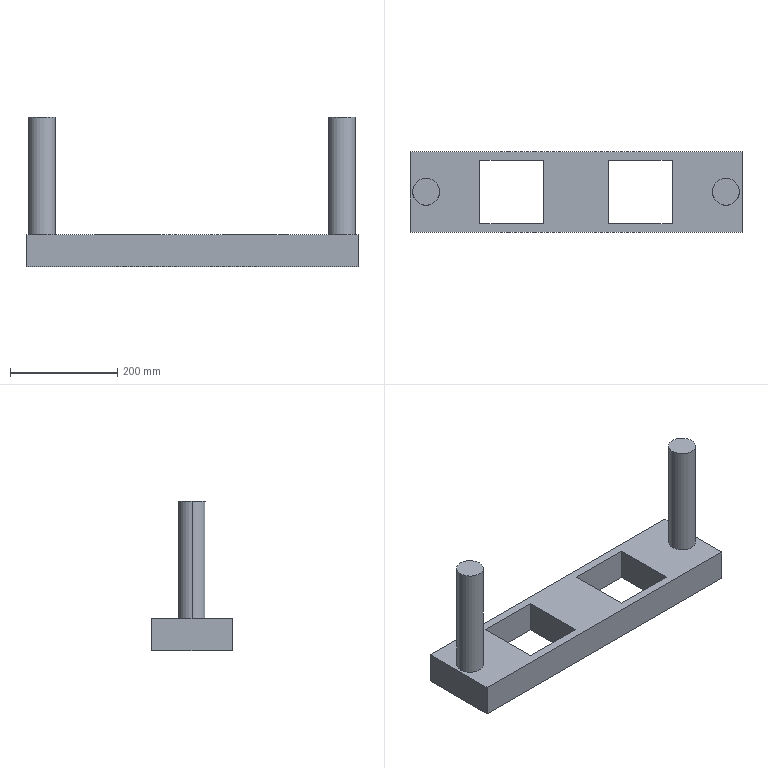Part | STEP file | 1 solid | 20 faces | box 620 x 150 x 280 mm | volume 4744618 mm3 | plane 16 | cylinder 4 | commonest cylinder face diameters 50 x4
STEP:
#1=CARTESIAN_POINT('',(0.,0.,0.));
#2=DIRECTION('',(0.,0.,1.));
#3=DIRECTION('',(1.,0.,0.));
#4=AXIS2_PLACEMENT_3D('',#1,#2,#3);
#5=CARTESIAN_POINT('',(-305.,0.,60.));
#6=VERTEX_POINT('',#5);
#7=CARTESIAN_POINT('',(-255.,0.,60.));
#8=VERTEX_POINT('',#7);
#9=CARTESIAN_POINT('',(-280.,0.,60.));
#10=DIRECTION('',(0.,0.,-1.));
#11=DIRECTION('',(1.,0.,0.));
#12=AXIS2_PLACEMENT_3D('',#9,#10,#11);
#13=CIRCLE('',#12,25.);
#14=CARTESIAN_POINT('',(-280.,0.,280.));
#15=DIRECTION('',(0.,0.,1.));
#16=DIRECTION('',(1.,0.,0.));
#17=AXIS2_PLACEMENT_3D('',#14,#15,#16);
#18=CYLINDRICAL_SURFACE('',#17,25.);
#19=CARTESIAN_POINT('',(6.283,-220.));
#20=DIRECTION('',(-1.,0.));
#21=VECTOR('',#20,1.);
#22=LINE('',#19,#21);
#23=(GEOMETRIC_REPRESENTATION_CONTEXT(2)PARAMETRIC_REPRESENTATION_CONTEXT()REPRESENTATION_CONTEXT('',''));
#24=DEFINITIONAL_REPRESENTATION('',(#22),#23);
#25=PCURVE('',#18,#24);
#26=CARTESIAN_POINT('',(0.,0.,60.));
#27=DIRECTION('',(0.,0.,1.));
#28=DIRECTION('',(1.,0.,0.));
#29=AXIS2_PLACEMENT_3D('',#26,#27,#28);
#30=PLANE('',#29);
#31=CARTESIAN_POINT('',(-255.,0.));
#32=CARTESIAN_POINT('',(-255.,-43.301));
#33=CARTESIAN_POINT('',(-292.5,-21.651));
#34=CARTESIAN_POINT('',(-330.,0.));
#35=CARTESIAN_POINT('',(-292.5,21.651));
#36=CARTESIAN_POINT('',(-255.,43.301));
#37=CARTESIAN_POINT('',(-255.,0.));
#38=(BOUNDED_CURVE()B_SPLINE_CURVE(2,(#31,#32,#33,#34,#35,#36,#37),.UNSPECIFIED.,.T.,.F.)B_SPLINE_CURVE_WITH_KNOTS((1,2,2,2,2,1),(-2.094,0.,2.094,4.189,6.283,8.378),.UNSPECIFIED.)CURVE()GEOMETRIC_REPRESENTATION_ITEM()RATIONAL_B_SPLINE_CURVE((1.,0.5,1.,0.5,1.,0.5,1.))REPRESENTATION_ITEM(''));
#39=(GEOMETRIC_REPRESENTATION_CONTEXT(2)PARAMETRIC_REPRESENTATION_CONTEXT()REPRESENTATION_CONTEXT('',''));
#40=DEFINITIONAL_REPRESENTATION('',(#38),#39);
#41=PCURVE('',#30,#40);
#42=SURFACE_CURVE('',#13,(#25,#41),.PCURVE_S1.);
#43=EDGE_CURVE('',#6,#8,#42,.T.);
#44=ORIENTED_EDGE('',*,*,#43,.F.);
#45=CARTESIAN_POINT('',(-305.,0.,280.));
#46=VERTEX_POINT('',#45);
#47=CARTESIAN_POINT('',(-305.,0.,280.));
#48=DIRECTION('',(0.,0.,1.));
#49=VECTOR('',#48,1.);
#50=LINE('',#47,#49);
#51=CARTESIAN_POINT('',(3.142,0.));
#52=DIRECTION('',(0.,1.));
#53=VECTOR('',#52,1.);
#54=LINE('',#51,#53);
#55=(GEOMETRIC_REPRESENTATION_CONTEXT(2)PARAMETRIC_REPRESENTATION_CONTEXT()REPRESENTATION_CONTEXT('',''));
#56=DEFINITIONAL_REPRESENTATION('',(#54),#55);
#57=PCURVE('',#18,#56);
#58=CARTESIAN_POINT('',(-280.,0.,280.));
#59=DIRECTION('',(0.,0.,1.));
#60=DIRECTION('',(1.,0.,0.));
#61=AXIS2_PLACEMENT_3D('',#58,#59,#60);
#62=CYLINDRICAL_SURFACE('',#61,25.);
#63=CARTESIAN_POINT('',(3.142,0.));
#64=DIRECTION('',(0.,1.));
#65=VECTOR('',#64,1.);
#66=LINE('',#63,#65);
#67=(GEOMETRIC_REPRESENTATION_CONTEXT(2)PARAMETRIC_REPRESENTATION_CONTEXT()REPRESENTATION_CONTEXT('',''));
#68=DEFINITIONAL_REPRESENTATION('',(#66),#67);
#69=PCURVE('',#62,#68);
#70=SURFACE_CURVE('',#50,(#57,#69),.PCURVE_S1.);
#71=EDGE_CURVE('',#6,#46,#70,.T.);
#72=ORIENTED_EDGE('',*,*,#71,.T.);
#73=CARTESIAN_POINT('',(-255.,0.,280.));
#74=VERTEX_POINT('',#73);
#75=CARTESIAN_POINT('',(-280.,0.,280.));
#76=DIRECTION('',(0.,0.,-1.));
#77=DIRECTION('',(1.,0.,0.));
#78=AXIS2_PLACEMENT_3D('',#75,#76,#77);
#79=CIRCLE('',#78,25.);
#80=CARTESIAN_POINT('',(6.283,0.));
#81=DIRECTION('',(-1.,0.));
#82=VECTOR('',#81,1.);
#83=LINE('',#80,#82);
#84=(GEOMETRIC_REPRESENTATION_CONTEXT(2)PARAMETRIC_REPRESENTATION_CONTEXT()REPRESENTATION_CONTEXT('',''));
#85=DEFINITIONAL_REPRESENTATION('',(#83),#84);
#86=PCURVE('',#18,#85);
#87=CARTESIAN_POINT('',(-280.,0.,280.));
#88=DIRECTION('',(0.,0.,1.));
#89=DIRECTION('',(1.,0.,0.));
#90=AXIS2_PLACEMENT_3D('',#87,#88,#89);
#91=PLANE('',#90);
#92=CARTESIAN_POINT('',(25.,0.));
#93=CARTESIAN_POINT('',(25.,-43.301));
#94=CARTESIAN_POINT('',(-12.5,-21.651));
#95=CARTESIAN_POINT('',(-50.,0.));
#96=CARTESIAN_POINT('',(-12.5,21.651));
#97=CARTESIAN_POINT('',(25.,43.301));
#98=CARTESIAN_POINT('',(25.,0.));
#99=(BOUNDED_CURVE()B_SPLINE_CURVE(2,(#92,#93,#94,#95,#96,#97,#98),.UNSPECIFIED.,.T.,.F.)B_SPLINE_CURVE_WITH_KNOTS((1,2,2,2,2,1),(-2.094,0.,2.094,4.189,6.283,8.378),.UNSPECIFIED.)CURVE()GEOMETRIC_REPRESENTATION_ITEM()RATIONAL_B_SPLINE_CURVE((1.,0.5,1.,0.5,1.,0.5,1.))REPRESENTATION_ITEM(''));
#100=(GEOMETRIC_REPRESENTATION_CONTEXT(2)PARAMETRIC_REPRESENTATION_CONTEXT()REPRESENTATION_CONTEXT('',''));
#101=DEFINITIONAL_REPRESENTATION('',(#99),#100);
#102=PCURVE('',#91,#101);
#103=SURFACE_CURVE('',#79,(#86,#102),.PCURVE_S1.);
#104=EDGE_CURVE('',#46,#74,#103,.T.);
#105=ORIENTED_EDGE('',*,*,#104,.T.);
#106=CARTESIAN_POINT('',(-255.,0.,280.));
#107=DIRECTION('',(0.,0.,1.));
#108=VECTOR('',#107,1.);
#109=LINE('',#106,#108);
#110=CARTESIAN_POINT('',(0.,0.));
#111=DIRECTION('',(0.,1.));
#112=VECTOR('',#111,1.);
#113=LINE('',#110,#112);
#114=(GEOMETRIC_REPRESENTATION_CONTEXT(2)PARAMETRIC_REPRESENTATION_CONTEXT()REPRESENTATION_CONTEXT('',''));
#115=DEFINITIONAL_REPRESENTATION('',(#113),#114);
#116=PCURVE('',#18,#115);
#117=CARTESIAN_POINT('',(6.283,0.));
#118=DIRECTION('',(0.,1.));
#119=VECTOR('',#118,1.);
#120=LINE('',#117,#119);
#121=(GEOMETRIC_REPRESENTATION_CONTEXT(2)PARAMETRIC_REPRESENTATION_CONTEXT()REPRESENTATION_CONTEXT('',''));
#122=DEFINITIONAL_REPRESENTATION('',(#120),#121);
#123=PCURVE('',#62,#122);
#124=SURFACE_CURVE('',#109,(#116,#123),.PCURVE_S1.);
#125=EDGE_CURVE('',#8,#74,#124,.T.);
#126=ORIENTED_EDGE('',*,*,#125,.F.);
#127=EDGE_LOOP('',(#44,#72,#105,#126));
#128=FACE_BOUND('',#127,.T.);
#129=ADVANCED_FACE('',(#128),#18,.T.);
#130=CARTESIAN_POINT('',(255.,0.,60.));
#131=VERTEX_POINT('',#130);
#132=CARTESIAN_POINT('',(305.,0.,60.));
#133=VERTEX_POINT('',#132);
#134=CARTESIAN_POINT('',(280.,0.,60.));
#135=DIRECTION('',(0.,0.,-1.));
#136=DIRECTION('',(1.,0.,0.));
#137=AXIS2_PLACEMENT_3D('',#134,#135,#136);
#138=CIRCLE('',#137,25.);
#139=CARTESIAN_POINT('',(280.,0.,280.));
#140=DIRECTION('',(0.,0.,1.));
#141=DIRECTION('',(1.,0.,0.));
#142=AXIS2_PLACEMENT_3D('',#139,#140,#141);
#143=CYLINDRICAL_SURFACE('',#142,25.);
#144=CARTESIAN_POINT('',(6.283,-220.));
#145=DIRECTION('',(-1.,0.));
#146=VECTOR('',#145,1.);
#147=LINE('',#144,#146);
#148=(GEOMETRIC_REPRESENTATION_CONTEXT(2)PARAMETRIC_REPRESENTATION_CONTEXT()REPRESENTATION_CONTEXT('',''));
#149=DEFINITIONAL_REPRESENTATION('',(#147),#148);
#150=PCURVE('',#143,#149);
#151=CARTESIAN_POINT('',(305.,0.));
#152=CARTESIAN_POINT('',(305.,-43.301));
#153=CARTESIAN_POINT('',(267.5,-21.651));
#154=CARTESIAN_POINT('',(230.,0.));
#155=CARTESIAN_POINT('',(267.5,21.651));
#156=CARTESIAN_POINT('',(305.,43.301));
#157=CARTESIAN_POINT('',(305.,0.));
#158=(BOUNDED_CURVE()B_SPLINE_CURVE(2,(#151,#152,#153,#154,#155,#156,#157),.UNSPECIFIED.,.T.,.F.)B_SPLINE_CURVE_WITH_KNOTS((1,2,2,2,2,1),(-2.094,0.,2.094,4.189,6.283,8.378),.UNSPECIFIED.)CURVE()GEOMETRIC_REPRESENTATION_ITEM()RATIONAL_B_SPLINE_CURVE((1.,0.5,1.,0.5,1.,0.5,1.))REPRESENTATION_ITEM(''));
#159=(GEOMETRIC_REPRESENTATION_CONTEXT(2)PARAMETRIC_REPRESENTATION_CONTEXT()REPRESENTATION_CONTEXT('',''));
#160=DEFINITIONAL_REPRESENTATION('',(#158),#159);
#161=PCURVE('',#30,#160);
#162=SURFACE_CURVE('',#138,(#150,#161),.PCURVE_S1.);
#163=EDGE_CURVE('',#131,#133,#162,.T.);
#164=ORIENTED_EDGE('',*,*,#163,.F.);
#165=CARTESIAN_POINT('',(255.,0.,280.));
#166=VERTEX_POINT('',#165);
#167=CARTESIAN_POINT('',(255.,0.,280.));
#168=DIRECTION('',(0.,0.,1.));
#169=VECTOR('',#168,1.);
#170=LINE('',#167,#169);
#171=CARTESIAN_POINT('',(3.142,0.));
#172=DIRECTION('',(0.,1.));
#173=VECTOR('',#172,1.);
#174=LINE('',#171,#173);
#175=(GEOMETRIC_REPRESENTATION_CONTEXT(2)PARAMETRIC_REPRESENTATION_CONTEXT()REPRESENTATION_CONTEXT('',''));
#176=DEFINITIONAL_REPRESENTATION('',(#174),#175);
#177=PCURVE('',#143,#176);
#178=CARTESIAN_POINT('',(280.,0.,280.));
#179=DIRECTION('',(0.,0.,1.));
#180=DIRECTION('',(1.,0.,0.));
#181=AXIS2_PLACEMENT_3D('',#178,#179,#180);
#182=CYLINDRICAL_SURFACE('',#181,25.);
#183=CARTESIAN_POINT('',(3.142,0.));
#184=DIRECTION('',(0.,1.));
#185=VECTOR('',#184,1.);
#186=LINE('',#183,#185);
#187=(GEOMETRIC_REPRESENTATION_CONTEXT(2)PARAMETRIC_REPRESENTATION_CONTEXT()REPRESENTATION_CONTEXT('',''));
#188=DEFINITIONAL_REPRESENTATION('',(#186),#187);
#189=PCURVE('',#182,#188);
#190=SURFACE_CURVE('',#170,(#177,#189),.PCURVE_S1.);
#191=EDGE_CURVE('',#131,#166,#190,.T.);
#192=ORIENTED_EDGE('',*,*,#191,.T.);
#193=CARTESIAN_POINT('',(305.,0.,280.));
#194=VERTEX_POINT('',#193);
#195=CARTESIAN_POINT('',(280.,0.,280.));
#196=DIRECTION('',(0.,0.,-1.));
#197=DIRECTION('',(1.,0.,0.));
#198=AXIS2_PLACEMENT_3D('',#195,#196,#197);
#199=CIRCLE('',#198,25.);
#200=CARTESIAN_POINT('',(6.283,0.));
#201=DIRECTION('',(-1.,0.));
#202=VECTOR('',#201,1.);
#203=LINE('',#200,#202);
#204=(GEOMETRIC_REPRESENTATION_CONTEXT(2)PARAMETRIC_REPRESENTATION_CONTEXT()REPRESENTATION_CONTEXT('',''));
#205=DEFINITIONAL_REPRESENTATION('',(#203),#204);
#206=PCURVE('',#143,#205);
#207=CARTESIAN_POINT('',(280.,0.,280.));
#208=DIRECTION('',(0.,0.,-1.));
#209=DIRECTION('',(-1.,0.,0.));
#210=AXIS2_PLACEMENT_3D('',#207,#208,#209);
#211=PLANE('',#210);
#212=CARTESIAN_POINT('',(0.,0.));
#213=DIRECTION('',(-1.,0.));
#214=AXIS2_PLACEMENT_2D('',#212,#213);
#215=CIRCLE('',#214,25.);
#216=(GEOMETRIC_REPRESENTATION_CONTEXT(2)PARAMETRIC_REPRESENTATION_CONTEXT()REPRESENTATION_CONTEXT('',''));
#217=DEFINITIONAL_REPRESENTATION('',(#215),#216);
#218=PCURVE('',#211,#217);
#219=SURFACE_CURVE('',#199,(#206,#218),.PCURVE_S1.);
#220=EDGE_CURVE('',#166,#194,#219,.T.);
#221=ORIENTED_EDGE('',*,*,#220,.T.);
#222=CARTESIAN_POINT('',(305.,0.,280.));
#223=DIRECTION('',(0.,0.,1.));
#224=VECTOR('',#223,1.);
#225=LINE('',#222,#224);
#226=CARTESIAN_POINT('',(0.,0.));
#227=DIRECTION('',(0.,1.));
#228=VECTOR('',#227,1.);
#229=LINE('',#226,#228);
#230=(GEOMETRIC_REPRESENTATION_CONTEXT(2)PARAMETRIC_REPRESENTATION_CONTEXT()REPRESENTATION_CONTEXT('',''));
#231=DEFINITIONAL_REPRESENTATION('',(#229),#230);
#232=PCURVE('',#143,#231);
#233=CARTESIAN_POINT('',(6.283,0.));
#234=DIRECTION('',(0.,1.));
#235=VECTOR('',#234,1.);
#236=LINE('',#233,#235);
#237=(GEOMETRIC_REPRESENTATION_CONTEXT(2)PARAMETRIC_REPRESENTATION_CONTEXT()REPRESENTATION_CONTEXT('',''));
#238=DEFINITIONAL_REPRESENTATION('',(#236),#237);
#239=PCURVE('',#182,#238);
#240=SURFACE_CURVE('',#225,(#232,#239),.PCURVE_S1.);
#241=EDGE_CURVE('',#133,#194,#240,.T.);
#242=ORIENTED_EDGE('',*,*,#241,.F.);
#243=EDGE_LOOP('',(#164,#192,#221,#242));
#244=FACE_BOUND('',#243,.T.);
#245=ADVANCED_FACE('',(#244),#143,.T.);
#246=CARTESIAN_POINT('',(60.5,-59.5,0.));
#247=VERTEX_POINT('',#246);
#248=CARTESIAN_POINT('',(60.5,59.5,0.));
#249=VERTEX_POINT('',#248);
#250=CARTESIAN_POINT('',(60.5,0.,0.));
#251=DIRECTION('',(0.,1.,0.));
#252=VECTOR('',#251,1.);
#253=LINE('',#250,#252);
#254=CARTESIAN_POINT('',(0.,0.,0.));
#255=DIRECTION('',(0.,0.,1.));
#256=DIRECTION('',(1.,0.,0.));
#257=AXIS2_PLACEMENT_3D('',#254,#255,#256);
#258=PLANE('',#257);
#259=CARTESIAN_POINT('',(60.5,0.));
#260=DIRECTION('',(0.,1.));
#261=VECTOR('',#260,1.);
#262=LINE('',#259,#261);
#263=(GEOMETRIC_REPRESENTATION_CONTEXT(2)PARAMETRIC_REPRESENTATION_CONTEXT()REPRESENTATION_CONTEXT('',''));
#264=DEFINITIONAL_REPRESENTATION('',(#262),#263);
#265=PCURVE('',#258,#264);
#266=CARTESIAN_POINT('',(60.5,59.5,400.));
#267=DIRECTION('',(-1.,0.,0.));
#268=DIRECTION('',(0.,-1.,0.));
#269=AXIS2_PLACEMENT_3D('',#266,#267,#268);
#270=PLANE('',#269);
#271=CARTESIAN_POINT('',(59.5,-400.));
#272=DIRECTION('',(-1.,0.));
#273=VECTOR('',#272,1.);
#274=LINE('',#271,#273);
#275=(GEOMETRIC_REPRESENTATION_CONTEXT(2)PARAMETRIC_REPRESENTATION_CONTEXT()REPRESENTATION_CONTEXT('',''));
#276=DEFINITIONAL_REPRESENTATION('',(#274),#275);
#277=PCURVE('',#270,#276);
#278=SURFACE_CURVE('',#253,(#265,#277),.PCURVE_S1.);
#279=EDGE_CURVE('',#247,#249,#278,.T.);
#280=ORIENTED_EDGE('',*,*,#279,.F.);
#281=CARTESIAN_POINT('',(179.5,-59.5,0.));
#282=VERTEX_POINT('',#281);
#283=CARTESIAN_POINT('',(0.,-59.5,0.));
#284=DIRECTION('',(-1.,0.,0.));
#285=VECTOR('',#284,1.);
#286=LINE('',#283,#285);
#287=CARTESIAN_POINT('',(0.,-59.5));
#288=DIRECTION('',(-1.,0.));
#289=VECTOR('',#288,1.);
#290=LINE('',#287,#289);
#291=(GEOMETRIC_REPRESENTATION_CONTEXT(2)PARAMETRIC_REPRESENTATION_CONTEXT()REPRESENTATION_CONTEXT('',''));
#292=DEFINITIONAL_REPRESENTATION('',(#290),#291);
#293=PCURVE('',#258,#292);
#294=CARTESIAN_POINT('',(179.5,-59.5,400.));
#295=DIRECTION('',(0.,-1.,0.));
#296=DIRECTION('',(0.,0.,-1.));
#297=AXIS2_PLACEMENT_3D('',#294,#295,#296);
#298=PLANE('',#297);
#299=CARTESIAN_POINT('',(400.,-179.5));
#300=DIRECTION('',(0.,-1.));
#301=VECTOR('',#300,1.);
#302=LINE('',#299,#301);
#303=(GEOMETRIC_REPRESENTATION_CONTEXT(2)PARAMETRIC_REPRESENTATION_CONTEXT()REPRESENTATION_CONTEXT('',''));
#304=DEFINITIONAL_REPRESENTATION('',(#302),#303);
#305=PCURVE('',#298,#304);
#306=SURFACE_CURVE('',#286,(#293,#305),.PCURVE_S1.);
#307=EDGE_CURVE('',#282,#247,#306,.T.);
#308=ORIENTED_EDGE('',*,*,#307,.F.);
#309=CARTESIAN_POINT('',(179.5,59.5,0.));
#310=VERTEX_POINT('',#309);
#311=CARTESIAN_POINT('',(179.5,0.,0.));
#312=DIRECTION('',(0.,-1.,0.));
#313=VECTOR('',#312,1.);
#314=LINE('',#311,#313);
#315=CARTESIAN_POINT('',(179.5,0.));
#316=DIRECTION('',(0.,-1.));
#317=VECTOR('',#316,1.);
#318=LINE('',#315,#317);
#319=(GEOMETRIC_REPRESENTATION_CONTEXT(2)PARAMETRIC_REPRESENTATION_CONTEXT()REPRESENTATION_CONTEXT('',''));
#320=DEFINITIONAL_REPRESENTATION('',(#318),#319);
#321=PCURVE('',#258,#320);
#322=CARTESIAN_POINT('',(179.5,59.5,400.));
#323=DIRECTION('',(1.,0.,0.));
#324=DIRECTION('',(0.,0.,-1.));
#325=AXIS2_PLACEMENT_3D('',#322,#323,#324);
#326=PLANE('',#325);
#327=CARTESIAN_POINT('',(400.,-59.5));
#328=DIRECTION('',(0.,-1.));
#329=VECTOR('',#328,1.);
#330=LINE('',#327,#329);
#331=(GEOMETRIC_REPRESENTATION_CONTEXT(2)PARAMETRIC_REPRESENTATION_CONTEXT()REPRESENTATION_CONTEXT('',''));
#332=DEFINITIONAL_REPRESENTATION('',(#330),#331);
#333=PCURVE('',#326,#332);
#334=SURFACE_CURVE('',#314,(#321,#333),.PCURVE_S1.);
#335=EDGE_CURVE('',#310,#282,#334,.T.);
#336=ORIENTED_EDGE('',*,*,#335,.F.);
#337=CARTESIAN_POINT('',(0.,59.5,0.));
#338=DIRECTION('',(1.,0.,0.));
#339=VECTOR('',#338,1.);
#340=LINE('',#337,#339);
#341=CARTESIAN_POINT('',(0.,59.5));
#342=DIRECTION('',(1.,0.));
#343=VECTOR('',#342,1.);
#344=LINE('',#341,#343);
#345=(GEOMETRIC_REPRESENTATION_CONTEXT(2)PARAMETRIC_REPRESENTATION_CONTEXT()REPRESENTATION_CONTEXT('',''));
#346=DEFINITIONAL_REPRESENTATION('',(#344),#345);
#347=PCURVE('',#258,#346);
#348=CARTESIAN_POINT('',(179.5,59.5,400.));
#349=DIRECTION('',(0.,1.,0.));
#350=DIRECTION('',(0.,0.,1.));
#351=AXIS2_PLACEMENT_3D('',#348,#349,#350);
#352=PLANE('',#351);
#353=CARTESIAN_POINT('',(-400.,-179.5));
#354=DIRECTION('',(0.,1.));
#355=VECTOR('',#354,1.);
#356=LINE('',#353,#355);
#357=(GEOMETRIC_REPRESENTATION_CONTEXT(2)PARAMETRIC_REPRESENTATION_CONTEXT()REPRESENTATION_CONTEXT('',''));
#358=DEFINITIONAL_REPRESENTATION('',(#356),#357);
#359=PCURVE('',#352,#358);
#360=SURFACE_CURVE('',#340,(#347,#359),.PCURVE_S1.);
#361=EDGE_CURVE('',#249,#310,#360,.T.);
#362=ORIENTED_EDGE('',*,*,#361,.F.);
#363=EDGE_LOOP('',(#280,#308,#336,#362));
#364=FACE_BOUND('',#363,.T.);
#365=CARTESIAN_POINT('',(-179.5,-59.5,0.));
#366=VERTEX_POINT('',#365);
#367=CARTESIAN_POINT('',(-179.5,59.5,0.));
#368=VERTEX_POINT('',#367);
#369=CARTESIAN_POINT('',(-179.5,0.,0.));
#370=DIRECTION('',(0.,1.,0.));
#371=VECTOR('',#370,1.);
#372=LINE('',#369,#371);
#373=CARTESIAN_POINT('',(-179.5,0.));
#374=DIRECTION('',(0.,1.));
#375=VECTOR('',#374,1.);
#376=LINE('',#373,#375);
#377=(GEOMETRIC_REPRESENTATION_CONTEXT(2)PARAMETRIC_REPRESENTATION_CONTEXT()REPRESENTATION_CONTEXT('',''));
#378=DEFINITIONAL_REPRESENTATION('',(#376),#377);
#379=PCURVE('',#258,#378);
#380=CARTESIAN_POINT('',(-179.5,59.5,400.));
#381=DIRECTION('',(-1.,0.,0.));
#382=DIRECTION('',(0.,0.,1.));
#383=AXIS2_PLACEMENT_3D('',#380,#381,#382);
#384=PLANE('',#383);
#385=CARTESIAN_POINT('',(-400.,-59.5));
#386=DIRECTION('',(0.,1.));
#387=VECTOR('',#386,1.);
#388=LINE('',#385,#387);
#389=(GEOMETRIC_REPRESENTATION_CONTEXT(2)PARAMETRIC_REPRESENTATION_CONTEXT()REPRESENTATION_CONTEXT('',''));
#390=DEFINITIONAL_REPRESENTATION('',(#388),#389);
#391=PCURVE('',#384,#390);
#392=SURFACE_CURVE('',#372,(#379,#391),.PCURVE_S1.);
#393=EDGE_CURVE('',#366,#368,#392,.T.);
#394=ORIENTED_EDGE('',*,*,#393,.F.);
#395=CARTESIAN_POINT('',(-60.5,-59.5,0.));
#396=VERTEX_POINT('',#395);
#397=CARTESIAN_POINT('',(0.,-59.5,0.));
#398=DIRECTION('',(-1.,0.,0.));
#399=VECTOR('',#398,1.);
#400=LINE('',#397,#399);
#401=CARTESIAN_POINT('',(0.,-59.5));
#402=DIRECTION('',(-1.,0.));
#403=VECTOR('',#402,1.);
#404=LINE('',#401,#403);
#405=(GEOMETRIC_REPRESENTATION_CONTEXT(2)PARAMETRIC_REPRESENTATION_CONTEXT()REPRESENTATION_CONTEXT('',''));
#406=DEFINITIONAL_REPRESENTATION('',(#404),#405);
#407=PCURVE('',#258,#406);
#408=CARTESIAN_POINT('',(-179.5,-59.5,400.));
#409=DIRECTION('',(0.,-1.,0.));
#410=DIRECTION('',(1.,0.,0.));
#411=AXIS2_PLACEMENT_3D('',#408,#409,#410);
#412=PLANE('',#411);
#413=CARTESIAN_POINT('',(179.5,-400.));
#414=DIRECTION('',(-1.,0.));
#415=VECTOR('',#414,1.);
#416=LINE('',#413,#415);
#417=(GEOMETRIC_REPRESENTATION_CONTEXT(2)PARAMETRIC_REPRESENTATION_CONTEXT()REPRESENTATION_CONTEXT('',''));
#418=DEFINITIONAL_REPRESENTATION('',(#416),#417);
#419=PCURVE('',#412,#418);
#420=SURFACE_CURVE('',#400,(#407,#419),.PCURVE_S1.);
#421=EDGE_CURVE('',#396,#366,#420,.T.);
#422=ORIENTED_EDGE('',*,*,#421,.F.);
#423=CARTESIAN_POINT('',(-60.5,59.5,0.));
#424=VERTEX_POINT('',#423);
#425=CARTESIAN_POINT('',(-60.5,0.,0.));
#426=DIRECTION('',(0.,-1.,0.));
#427=VECTOR('',#426,1.);
#428=LINE('',#425,#427);
#429=CARTESIAN_POINT('',(-60.5,0.));
#430=DIRECTION('',(0.,-1.));
#431=VECTOR('',#430,1.);
#432=LINE('',#429,#431);
#433=(GEOMETRIC_REPRESENTATION_CONTEXT(2)PARAMETRIC_REPRESENTATION_CONTEXT()REPRESENTATION_CONTEXT('',''));
#434=DEFINITIONAL_REPRESENTATION('',(#432),#433);
#435=PCURVE('',#258,#434);
#436=CARTESIAN_POINT('',(-60.5,59.5,400.));
#437=DIRECTION('',(1.,0.,0.));
#438=DIRECTION('',(0.,1.,0.));
#439=AXIS2_PLACEMENT_3D('',#436,#437,#438);
#440=PLANE('',#439);
#441=CARTESIAN_POINT('',(-59.5,-400.));
#442=DIRECTION('',(-1.,0.));
#443=VECTOR('',#442,1.);
#444=LINE('',#441,#443);
#445=(GEOMETRIC_REPRESENTATION_CONTEXT(2)PARAMETRIC_REPRESENTATION_CONTEXT()REPRESENTATION_CONTEXT('',''));
#446=DEFINITIONAL_REPRESENTATION('',(#444),#445);
#447=PCURVE('',#440,#446);
#448=SURFACE_CURVE('',#428,(#435,#447),.PCURVE_S1.);
#449=EDGE_CURVE('',#424,#396,#448,.T.);
#450=ORIENTED_EDGE('',*,*,#449,.F.);
#451=CARTESIAN_POINT('',(0.,59.5,0.));
#452=DIRECTION('',(1.,0.,0.));
#453=VECTOR('',#452,1.);
#454=LINE('',#451,#453);
#455=CARTESIAN_POINT('',(0.,59.5));
#456=DIRECTION('',(1.,0.));
#457=VECTOR('',#456,1.);
#458=LINE('',#455,#457);
#459=(GEOMETRIC_REPRESENTATION_CONTEXT(2)PARAMETRIC_REPRESENTATION_CONTEXT()REPRESENTATION_CONTEXT('',''));
#460=DEFINITIONAL_REPRESENTATION('',(#458),#459);
#461=PCURVE('',#258,#460);
#462=CARTESIAN_POINT('',(-179.5,59.5,400.));
#463=DIRECTION('',(0.,1.,0.));
#464=DIRECTION('',(-1.,0.,0.));
#465=AXIS2_PLACEMENT_3D('',#462,#463,#464);
#466=PLANE('',#465);
#467=CARTESIAN_POINT('',(-179.5,-400.));
#468=DIRECTION('',(-1.,0.));
#469=VECTOR('',#468,1.);
#470=LINE('',#467,#469);
#471=(GEOMETRIC_REPRESENTATION_CONTEXT(2)PARAMETRIC_REPRESENTATION_CONTEXT()REPRESENTATION_CONTEXT('',''));
#472=DEFINITIONAL_REPRESENTATION('',(#470),#471);
#473=PCURVE('',#466,#472);
#474=SURFACE_CURVE('',#454,(#461,#473),.PCURVE_S1.);
#475=EDGE_CURVE('',#368,#424,#474,.T.);
#476=ORIENTED_EDGE('',*,*,#475,.F.);
#477=EDGE_LOOP('',(#394,#422,#450,#476));
#478=FACE_BOUND('',#477,.T.);
#479=CARTESIAN_POINT('',(-310.,-75.,0.));
#480=VERTEX_POINT('',#479);
#481=CARTESIAN_POINT('',(310.,-75.,0.));
#482=VERTEX_POINT('',#481);
#483=CARTESIAN_POINT('',(0.,-75.,0.));
#484=DIRECTION('',(1.,0.,0.));
#485=VECTOR('',#484,1.);
#486=LINE('',#483,#485);
#487=CARTESIAN_POINT('',(0.,-75.));
#488=DIRECTION('',(1.,0.));
#489=VECTOR('',#488,1.);
#490=LINE('',#487,#489);
#491=(GEOMETRIC_REPRESENTATION_CONTEXT(2)PARAMETRIC_REPRESENTATION_CONTEXT()REPRESENTATION_CONTEXT('',''));
#492=DEFINITIONAL_REPRESENTATION('',(#490),#491);
#493=PCURVE('',#258,#492);
#494=CARTESIAN_POINT('',(-310.,-75.,60.));
#495=DIRECTION('',(0.,1.,0.));
#496=DIRECTION('',(0.,0.,1.));
#497=AXIS2_PLACEMENT_3D('',#494,#495,#496);
#498=PLANE('',#497);
#499=CARTESIAN_POINT('',(-60.,310.));
#500=DIRECTION('',(0.,1.));
#501=VECTOR('',#500,1.);
#502=LINE('',#499,#501);
#503=(GEOMETRIC_REPRESENTATION_CONTEXT(2)PARAMETRIC_REPRESENTATION_CONTEXT()REPRESENTATION_CONTEXT('',''));
#504=DEFINITIONAL_REPRESENTATION('',(#502),#503);
#505=PCURVE('',#498,#504);
#506=SURFACE_CURVE('',#486,(#493,#505),.PCURVE_S1.);
#507=EDGE_CURVE('',#480,#482,#506,.T.);
#508=ORIENTED_EDGE('',*,*,#507,.F.);
#509=CARTESIAN_POINT('',(-310.,75.,0.));
#510=VERTEX_POINT('',#509);
#511=CARTESIAN_POINT('',(-310.,0.,0.));
#512=DIRECTION('',(0.,-1.,0.));
#513=VECTOR('',#512,1.);
#514=LINE('',#511,#513);
#515=CARTESIAN_POINT('',(-310.,0.));
#516=DIRECTION('',(0.,-1.));
#517=VECTOR('',#516,1.);
#518=LINE('',#515,#517);
#519=(GEOMETRIC_REPRESENTATION_CONTEXT(2)PARAMETRIC_REPRESENTATION_CONTEXT()REPRESENTATION_CONTEXT('',''));
#520=DEFINITIONAL_REPRESENTATION('',(#518),#519);
#521=PCURVE('',#258,#520);
#522=CARTESIAN_POINT('',(-310.,75.,60.));
#523=DIRECTION('',(1.,0.,0.));
#524=DIRECTION('',(0.,0.,-1.));
#525=AXIS2_PLACEMENT_3D('',#522,#523,#524);
#526=PLANE('',#525);
#527=CARTESIAN_POINT('',(60.,-75.));
#528=DIRECTION('',(0.,-1.));
#529=VECTOR('',#528,1.);
#530=LINE('',#527,#529);
#531=(GEOMETRIC_REPRESENTATION_CONTEXT(2)PARAMETRIC_REPRESENTATION_CONTEXT()REPRESENTATION_CONTEXT('',''));
#532=DEFINITIONAL_REPRESENTATION('',(#530),#531);
#533=PCURVE('',#526,#532);
#534=SURFACE_CURVE('',#514,(#521,#533),.PCURVE_S1.);
#535=EDGE_CURVE('',#510,#480,#534,.T.);
#536=ORIENTED_EDGE('',*,*,#535,.F.);
#537=CARTESIAN_POINT('',(310.,75.,0.));
#538=VERTEX_POINT('',#537);
#539=CARTESIAN_POINT('',(0.,75.,0.));
#540=DIRECTION('',(-1.,0.,0.));
#541=VECTOR('',#540,1.);
#542=LINE('',#539,#541);
#543=CARTESIAN_POINT('',(0.,75.));
#544=DIRECTION('',(-1.,0.));
#545=VECTOR('',#544,1.);
#546=LINE('',#543,#545);
#547=(GEOMETRIC_REPRESENTATION_CONTEXT(2)PARAMETRIC_REPRESENTATION_CONTEXT()REPRESENTATION_CONTEXT('',''));
#548=DEFINITIONAL_REPRESENTATION('',(#546),#547);
#549=PCURVE('',#258,#548);
#550=CARTESIAN_POINT('',(-310.,75.,60.));
#551=DIRECTION('',(0.,-1.,0.));
#552=DIRECTION('',(0.,0.,-1.));
#553=AXIS2_PLACEMENT_3D('',#550,#551,#552);
#554=PLANE('',#553);
#555=CARTESIAN_POINT('',(60.,310.));
#556=DIRECTION('',(0.,-1.));
#557=VECTOR('',#556,1.);
#558=LINE('',#555,#557);
#559=(GEOMETRIC_REPRESENTATION_CONTEXT(2)PARAMETRIC_REPRESENTATION_CONTEXT()REPRESENTATION_CONTEXT('',''));
#560=DEFINITIONAL_REPRESENTATION('',(#558),#559);
#561=PCURVE('',#554,#560);
#562=SURFACE_CURVE('',#542,(#549,#561),.PCURVE_S1.);
#563=EDGE_CURVE('',#538,#510,#562,.T.);
#564=ORIENTED_EDGE('',*,*,#563,.F.);
#565=CARTESIAN_POINT('',(310.,0.,0.));
#566=DIRECTION('',(0.,1.,0.));
#567=VECTOR('',#566,1.);
#568=LINE('',#565,#567);
#569=CARTESIAN_POINT('',(310.,0.));
#570=DIRECTION('',(0.,1.));
#571=VECTOR('',#570,1.);
#572=LINE('',#569,#571);
#573=(GEOMETRIC_REPRESENTATION_CONTEXT(2)PARAMETRIC_REPRESENTATION_CONTEXT()REPRESENTATION_CONTEXT('',''));
#574=DEFINITIONAL_REPRESENTATION('',(#572),#573);
#575=PCURVE('',#258,#574);
#576=CARTESIAN_POINT('',(310.,75.,60.));
#577=DIRECTION('',(-1.,0.,0.));
#578=DIRECTION('',(0.,-1.,0.));
#579=AXIS2_PLACEMENT_3D('',#576,#577,#578);
#580=PLANE('',#579);
#581=CARTESIAN_POINT('',(75.,-60.));
#582=DIRECTION('',(-1.,0.));
#583=VECTOR('',#582,1.);
#584=LINE('',#581,#583);
#585=(GEOMETRIC_REPRESENTATION_CONTEXT(2)PARAMETRIC_REPRESENTATION_CONTEXT()REPRESENTATION_CONTEXT('',''));
#586=DEFINITIONAL_REPRESENTATION('',(#584),#585);
#587=PCURVE('',#580,#586);
#588=SURFACE_CURVE('',#568,(#575,#587),.PCURVE_S1.);
#589=EDGE_CURVE('',#482,#538,#588,.T.);
#590=ORIENTED_EDGE('',*,*,#589,.F.);
#591=EDGE_LOOP('',(#508,#536,#564,#590));
#592=FACE_BOUND('',#591,.T.);
#593=ADVANCED_FACE('',(#364,#478,#592),#258,.F.);
#594=CARTESIAN_POINT('',(60.5,59.5,60.));
#595=VERTEX_POINT('',#594);
#596=CARTESIAN_POINT('',(60.5,59.5,400.));
#597=DIRECTION('',(0.,0.,1.));
#598=VECTOR('',#597,1.);
#599=LINE('',#596,#598);
#600=CARTESIAN_POINT('',(0.,-119.));
#601=DIRECTION('',(1.,0.));
#602=VECTOR('',#601,1.);
#603=LINE('',#600,#602);
#604=(GEOMETRIC_REPRESENTATION_CONTEXT(2)PARAMETRIC_REPRESENTATION_CONTEXT()REPRESENTATION_CONTEXT('',''));
#605=DEFINITIONAL_REPRESENTATION('',(#603),#604);
#606=PCURVE('',#352,#605);
#607=CARTESIAN_POINT('',(0.,0.));
#608=DIRECTION('',(0.,1.));
#609=VECTOR('',#608,1.);
#610=LINE('',#607,#609);
#611=(GEOMETRIC_REPRESENTATION_CONTEXT(2)PARAMETRIC_REPRESENTATION_CONTEXT()REPRESENTATION_CONTEXT('',''));
#612=DEFINITIONAL_REPRESENTATION('',(#610),#611);
#613=PCURVE('',#270,#612);
#614=SURFACE_CURVE('',#599,(#606,#613),.PCURVE_S1.);
#615=EDGE_CURVE('',#249,#595,#614,.T.);
#616=ORIENTED_EDGE('',*,*,#615,.F.);
#617=ORIENTED_EDGE('',*,*,#361,.T.);
#618=CARTESIAN_POINT('',(179.5,59.5,60.));
#619=VERTEX_POINT('',#618);
#620=CARTESIAN_POINT('',(179.5,59.5,400.));
#621=DIRECTION('',(0.,0.,-1.));
#622=VECTOR('',#621,1.);
#623=LINE('',#620,#622);
#624=CARTESIAN_POINT('',(0.,0.));
#625=DIRECTION('',(-1.,0.));
#626=VECTOR('',#625,1.);
#627=LINE('',#624,#626);
#628=(GEOMETRIC_REPRESENTATION_CONTEXT(2)PARAMETRIC_REPRESENTATION_CONTEXT()REPRESENTATION_CONTEXT('',''));
#629=DEFINITIONAL_REPRESENTATION('',(#627),#628);
#630=PCURVE('',#352,#629);
#631=CARTESIAN_POINT('',(0.,0.));
#632=DIRECTION('',(1.,0.));
#633=VECTOR('',#632,1.);
#634=LINE('',#631,#633);
#635=(GEOMETRIC_REPRESENTATION_CONTEXT(2)PARAMETRIC_REPRESENTATION_CONTEXT()REPRESENTATION_CONTEXT('',''));
#636=DEFINITIONAL_REPRESENTATION('',(#634),#635);
#637=PCURVE('',#326,#636);
#638=SURFACE_CURVE('',#623,(#630,#637),.PCURVE_S1.);
#639=EDGE_CURVE('',#619,#310,#638,.T.);
#640=ORIENTED_EDGE('',*,*,#639,.F.);
#641=CARTESIAN_POINT('',(179.5,59.5,60.));
#642=DIRECTION('',(1.,0.,0.));
#643=VECTOR('',#642,1.);
#644=LINE('',#641,#643);
#645=CARTESIAN_POINT('',(-340.,0.));
#646=DIRECTION('',(0.,1.));
#647=VECTOR('',#646,1.);
#648=LINE('',#645,#647);
#649=(GEOMETRIC_REPRESENTATION_CONTEXT(2)PARAMETRIC_REPRESENTATION_CONTEXT()REPRESENTATION_CONTEXT('',''));
#650=DEFINITIONAL_REPRESENTATION('',(#648),#649);
#651=PCURVE('',#352,#650);
#652=CARTESIAN_POINT('',(179.5,59.5));
#653=DIRECTION('',(1.,0.));
#654=VECTOR('',#653,1.);
#655=LINE('',#652,#654);
#656=(GEOMETRIC_REPRESENTATION_CONTEXT(2)PARAMETRIC_REPRESENTATION_CONTEXT()REPRESENTATION_CONTEXT('',''));
#657=DEFINITIONAL_REPRESENTATION('',(#655),#656);
#658=PCURVE('',#30,#657);
#659=SURFACE_CURVE('',#644,(#651,#658),.PCURVE_S1.);
#660=EDGE_CURVE('',#595,#619,#659,.T.);
#661=ORIENTED_EDGE('',*,*,#660,.F.);
#662=EDGE_LOOP('',(#616,#617,#640,#661));
#663=FACE_BOUND('',#662,.T.);
#664=ADVANCED_FACE('',(#663),#352,.F.);
#665=CARTESIAN_POINT('',(60.5,-59.5,60.));
#666=VERTEX_POINT('',#665);
#667=CARTESIAN_POINT('',(60.5,-59.5,400.));
#668=DIRECTION('',(0.,0.,1.));
#669=VECTOR('',#668,1.);
#670=LINE('',#667,#669);
#671=CARTESIAN_POINT('',(119.,0.));
#672=DIRECTION('',(0.,1.));
#673=VECTOR('',#672,1.);
#674=LINE('',#671,#673);
#675=(GEOMETRIC_REPRESENTATION_CONTEXT(2)PARAMETRIC_REPRESENTATION_CONTEXT()REPRESENTATION_CONTEXT('',''));
#676=DEFINITIONAL_REPRESENTATION('',(#674),#675);
#677=PCURVE('',#270,#676);
#678=CARTESIAN_POINT('',(0.,-119.));
#679=DIRECTION('',(-1.,0.));
#680=VECTOR('',#679,1.);
#681=LINE('',#678,#680);
#682=(GEOMETRIC_REPRESENTATION_CONTEXT(2)PARAMETRIC_REPRESENTATION_CONTEXT()REPRESENTATION_CONTEXT('',''));
#683=DEFINITIONAL_REPRESENTATION('',(#681),#682);
#684=PCURVE('',#298,#683);
#685=SURFACE_CURVE('',#670,(#677,#684),.PCURVE_S1.);
#686=EDGE_CURVE('',#247,#666,#685,.T.);
#687=ORIENTED_EDGE('',*,*,#686,.F.);
#688=ORIENTED_EDGE('',*,*,#279,.T.);
#689=ORIENTED_EDGE('',*,*,#615,.T.);
#690=CARTESIAN_POINT('',(60.5,59.5,60.));
#691=DIRECTION('',(0.,1.,0.));
#692=VECTOR('',#691,1.);
#693=LINE('',#690,#692);
#694=CARTESIAN_POINT('',(0.,-340.));
#695=DIRECTION('',(-1.,0.));
#696=VECTOR('',#695,1.);
#697=LINE('',#694,#696);
#698=(GEOMETRIC_REPRESENTATION_CONTEXT(2)PARAMETRIC_REPRESENTATION_CONTEXT()REPRESENTATION_CONTEXT('',''));
#699=DEFINITIONAL_REPRESENTATION('',(#697),#698);
#700=PCURVE('',#270,#699);
#701=CARTESIAN_POINT('',(60.5,59.5));
#702=DIRECTION('',(0.,1.));
#703=VECTOR('',#702,1.);
#704=LINE('',#701,#703);
#705=(GEOMETRIC_REPRESENTATION_CONTEXT(2)PARAMETRIC_REPRESENTATION_CONTEXT()REPRESENTATION_CONTEXT('',''));
#706=DEFINITIONAL_REPRESENTATION('',(#704),#705);
#707=PCURVE('',#30,#706);
#708=SURFACE_CURVE('',#693,(#700,#707),.PCURVE_S1.);
#709=EDGE_CURVE('',#666,#595,#708,.T.);
#710=ORIENTED_EDGE('',*,*,#709,.F.);
#711=EDGE_LOOP('',(#687,#688,#689,#710));
#712=FACE_BOUND('',#711,.T.);
#713=ADVANCED_FACE('',(#712),#270,.F.);
#714=CARTESIAN_POINT('',(179.5,-59.5,60.));
#715=VERTEX_POINT('',#714);
#716=CARTESIAN_POINT('',(179.5,-59.5,400.));
#717=DIRECTION('',(0.,0.,1.));
#718=VECTOR('',#717,1.);
#719=LINE('',#716,#718);
#720=CARTESIAN_POINT('',(0.,0.));
#721=DIRECTION('',(-1.,0.));
#722=VECTOR('',#721,1.);
#723=LINE('',#720,#722);
#724=(GEOMETRIC_REPRESENTATION_CONTEXT(2)PARAMETRIC_REPRESENTATION_CONTEXT()REPRESENTATION_CONTEXT('',''));
#725=DEFINITIONAL_REPRESENTATION('',(#723),#724);
#726=PCURVE('',#298,#725);
#727=CARTESIAN_POINT('',(0.,-119.));
#728=DIRECTION('',(-1.,0.));
#729=VECTOR('',#728,1.);
#730=LINE('',#727,#729);
#731=(GEOMETRIC_REPRESENTATION_CONTEXT(2)PARAMETRIC_REPRESENTATION_CONTEXT()REPRESENTATION_CONTEXT('',''));
#732=DEFINITIONAL_REPRESENTATION('',(#730),#731);
#733=PCURVE('',#326,#732);
#734=SURFACE_CURVE('',#719,(#726,#733),.PCURVE_S1.);
#735=EDGE_CURVE('',#282,#715,#734,.T.);
#736=ORIENTED_EDGE('',*,*,#735,.F.);
#737=ORIENTED_EDGE('',*,*,#307,.T.);
#738=ORIENTED_EDGE('',*,*,#686,.T.);
#739=CARTESIAN_POINT('',(179.5,-59.5,60.));
#740=DIRECTION('',(-1.,0.,0.));
#741=VECTOR('',#740,1.);
#742=LINE('',#739,#741);
#743=CARTESIAN_POINT('',(340.,0.));
#744=DIRECTION('',(0.,-1.));
#745=VECTOR('',#744,1.);
#746=LINE('',#743,#745);
#747=(GEOMETRIC_REPRESENTATION_CONTEXT(2)PARAMETRIC_REPRESENTATION_CONTEXT()REPRESENTATION_CONTEXT('',''));
#748=DEFINITIONAL_REPRESENTATION('',(#746),#747);
#749=PCURVE('',#298,#748);
#750=CARTESIAN_POINT('',(179.5,-59.5));
#751=DIRECTION('',(-1.,0.));
#752=VECTOR('',#751,1.);
#753=LINE('',#750,#752);
#754=(GEOMETRIC_REPRESENTATION_CONTEXT(2)PARAMETRIC_REPRESENTATION_CONTEXT()REPRESENTATION_CONTEXT('',''));
#755=DEFINITIONAL_REPRESENTATION('',(#753),#754);
#756=PCURVE('',#30,#755);
#757=SURFACE_CURVE('',#742,(#749,#756),.PCURVE_S1.);
#758=EDGE_CURVE('',#715,#666,#757,.T.);
#759=ORIENTED_EDGE('',*,*,#758,.F.);
#760=EDGE_LOOP('',(#736,#737,#738,#759));
#761=FACE_BOUND('',#760,.T.);
#762=ADVANCED_FACE('',(#761),#298,.F.);
#763=ORIENTED_EDGE('',*,*,#639,.T.);
#764=ORIENTED_EDGE('',*,*,#335,.T.);
#765=ORIENTED_EDGE('',*,*,#735,.T.);
#766=CARTESIAN_POINT('',(179.5,59.5,60.));
#767=DIRECTION('',(0.,-1.,0.));
#768=VECTOR('',#767,1.);
#769=LINE('',#766,#768);
#770=CARTESIAN_POINT('',(340.,0.));
#771=DIRECTION('',(0.,-1.));
#772=VECTOR('',#771,1.);
#773=LINE('',#770,#772);
#774=(GEOMETRIC_REPRESENTATION_CONTEXT(2)PARAMETRIC_REPRESENTATION_CONTEXT()REPRESENTATION_CONTEXT('',''));
#775=DEFINITIONAL_REPRESENTATION('',(#773),#774);
#776=PCURVE('',#326,#775);
#777=CARTESIAN_POINT('',(179.5,59.5));
#778=DIRECTION('',(0.,-1.));
#779=VECTOR('',#778,1.);
#780=LINE('',#777,#779);
#781=(GEOMETRIC_REPRESENTATION_CONTEXT(2)PARAMETRIC_REPRESENTATION_CONTEXT()REPRESENTATION_CONTEXT('',''));
#782=DEFINITIONAL_REPRESENTATION('',(#780),#781);
#783=PCURVE('',#30,#782);
#784=SURFACE_CURVE('',#769,(#776,#783),.PCURVE_S1.);
#785=EDGE_CURVE('',#619,#715,#784,.T.);
#786=ORIENTED_EDGE('',*,*,#785,.F.);
#787=EDGE_LOOP('',(#763,#764,#765,#786));
#788=FACE_BOUND('',#787,.T.);
#789=ADVANCED_FACE('',(#788),#326,.F.);
#790=CARTESIAN_POINT('',(-179.5,59.5,60.));
#791=VERTEX_POINT('',#790);
#792=CARTESIAN_POINT('',(-179.5,59.5,400.));
#793=DIRECTION('',(0.,0.,1.));
#794=VECTOR('',#793,1.);
#795=LINE('',#792,#794);
#796=CARTESIAN_POINT('',(0.,0.));
#797=DIRECTION('',(0.,1.));
#798=VECTOR('',#797,1.);
#799=LINE('',#796,#798);
#800=(GEOMETRIC_REPRESENTATION_CONTEXT(2)PARAMETRIC_REPRESENTATION_CONTEXT()REPRESENTATION_CONTEXT('',''));
#801=DEFINITIONAL_REPRESENTATION('',(#799),#800);
#802=PCURVE('',#466,#801);
#803=CARTESIAN_POINT('',(0.,0.));
#804=DIRECTION('',(1.,0.));
#805=VECTOR('',#804,1.);
#806=LINE('',#803,#805);
#807=(GEOMETRIC_REPRESENTATION_CONTEXT(2)PARAMETRIC_REPRESENTATION_CONTEXT()REPRESENTATION_CONTEXT('',''));
#808=DEFINITIONAL_REPRESENTATION('',(#806),#807);
#809=PCURVE('',#384,#808);
#810=SURFACE_CURVE('',#795,(#802,#809),.PCURVE_S1.);
#811=EDGE_CURVE('',#368,#791,#810,.T.);
#812=ORIENTED_EDGE('',*,*,#811,.F.);
#813=ORIENTED_EDGE('',*,*,#475,.T.);
#814=CARTESIAN_POINT('',(-60.5,59.5,60.));
#815=VERTEX_POINT('',#814);
#816=CARTESIAN_POINT('',(-60.5,59.5,400.));
#817=DIRECTION('',(0.,0.,-1.));
#818=VECTOR('',#817,1.);
#819=LINE('',#816,#818);
#820=CARTESIAN_POINT('',(-119.,0.));
#821=DIRECTION('',(0.,-1.));
#822=VECTOR('',#821,1.);
#823=LINE('',#820,#822);
#824=(GEOMETRIC_REPRESENTATION_CONTEXT(2)PARAMETRIC_REPRESENTATION_CONTEXT()REPRESENTATION_CONTEXT('',''));
#825=DEFINITIONAL_REPRESENTATION('',(#823),#824);
#826=PCURVE('',#466,#825);
#827=CARTESIAN_POINT('',(0.,0.));
#828=DIRECTION('',(0.,-1.));
#829=VECTOR('',#828,1.);
#830=LINE('',#827,#829);
#831=(GEOMETRIC_REPRESENTATION_CONTEXT(2)PARAMETRIC_REPRESENTATION_CONTEXT()REPRESENTATION_CONTEXT('',''));
#832=DEFINITIONAL_REPRESENTATION('',(#830),#831);
#833=PCURVE('',#440,#832);
#834=SURFACE_CURVE('',#819,(#826,#833),.PCURVE_S1.);
#835=EDGE_CURVE('',#815,#424,#834,.T.);
#836=ORIENTED_EDGE('',*,*,#835,.F.);
#837=CARTESIAN_POINT('',(-179.5,59.5,60.));
#838=DIRECTION('',(1.,0.,0.));
#839=VECTOR('',#838,1.);
#840=LINE('',#837,#839);
#841=CARTESIAN_POINT('',(0.,-340.));
#842=DIRECTION('',(-1.,0.));
#843=VECTOR('',#842,1.);
#844=LINE('',#841,#843);
#845=(GEOMETRIC_REPRESENTATION_CONTEXT(2)PARAMETRIC_REPRESENTATION_CONTEXT()REPRESENTATION_CONTEXT('',''));
#846=DEFINITIONAL_REPRESENTATION('',(#844),#845);
#847=PCURVE('',#466,#846);
#848=CARTESIAN_POINT('',(-179.5,59.5));
#849=DIRECTION('',(1.,0.));
#850=VECTOR('',#849,1.);
#851=LINE('',#848,#850);
#852=(GEOMETRIC_REPRESENTATION_CONTEXT(2)PARAMETRIC_REPRESENTATION_CONTEXT()REPRESENTATION_CONTEXT('',''));
#853=DEFINITIONAL_REPRESENTATION('',(#851),#852);
#854=PCURVE('',#30,#853);
#855=SURFACE_CURVE('',#840,(#847,#854),.PCURVE_S1.);
#856=EDGE_CURVE('',#791,#815,#855,.T.);
#857=ORIENTED_EDGE('',*,*,#856,.F.);
#858=EDGE_LOOP('',(#812,#813,#836,#857));
#859=FACE_BOUND('',#858,.T.);
#860=ADVANCED_FACE('',(#859),#466,.F.);
#861=CARTESIAN_POINT('',(-179.5,-59.5,60.));
#862=VERTEX_POINT('',#861);
#863=CARTESIAN_POINT('',(-179.5,-59.5,400.));
#864=DIRECTION('',(0.,0.,1.));
#865=VECTOR('',#864,1.);
#866=LINE('',#863,#865);
#867=CARTESIAN_POINT('',(0.,-119.));
#868=DIRECTION('',(1.,0.));
#869=VECTOR('',#868,1.);
#870=LINE('',#867,#869);
#871=(GEOMETRIC_REPRESENTATION_CONTEXT(2)PARAMETRIC_REPRESENTATION_CONTEXT()REPRESENTATION_CONTEXT('',''));
#872=DEFINITIONAL_REPRESENTATION('',(#870),#871);
#873=PCURVE('',#384,#872);
#874=CARTESIAN_POINT('',(0.,0.));
#875=DIRECTION('',(0.,1.));
#876=VECTOR('',#875,1.);
#877=LINE('',#874,#876);
#878=(GEOMETRIC_REPRESENTATION_CONTEXT(2)PARAMETRIC_REPRESENTATION_CONTEXT()REPRESENTATION_CONTEXT('',''));
#879=DEFINITIONAL_REPRESENTATION('',(#877),#878);
#880=PCURVE('',#412,#879);
#881=SURFACE_CURVE('',#866,(#873,#880),.PCURVE_S1.);
#882=EDGE_CURVE('',#366,#862,#881,.T.);
#883=ORIENTED_EDGE('',*,*,#882,.F.);
#884=ORIENTED_EDGE('',*,*,#393,.T.);
#885=ORIENTED_EDGE('',*,*,#811,.T.);
#886=CARTESIAN_POINT('',(-179.5,59.5,60.));
#887=DIRECTION('',(0.,1.,0.));
#888=VECTOR('',#887,1.);
#889=LINE('',#886,#888);
#890=CARTESIAN_POINT('',(-340.,0.));
#891=DIRECTION('',(0.,1.));
#892=VECTOR('',#891,1.);
#893=LINE('',#890,#892);
#894=(GEOMETRIC_REPRESENTATION_CONTEXT(2)PARAMETRIC_REPRESENTATION_CONTEXT()REPRESENTATION_CONTEXT('',''));
#895=DEFINITIONAL_REPRESENTATION('',(#893),#894);
#896=PCURVE('',#384,#895);
#897=CARTESIAN_POINT('',(-179.5,59.5));
#898=DIRECTION('',(0.,1.));
#899=VECTOR('',#898,1.);
#900=LINE('',#897,#899);
#901=(GEOMETRIC_REPRESENTATION_CONTEXT(2)PARAMETRIC_REPRESENTATION_CONTEXT()REPRESENTATION_CONTEXT('',''));
#902=DEFINITIONAL_REPRESENTATION('',(#900),#901);
#903=PCURVE('',#30,#902);
#904=SURFACE_CURVE('',#889,(#896,#903),.PCURVE_S1.);
#905=EDGE_CURVE('',#862,#791,#904,.T.);
#906=ORIENTED_EDGE('',*,*,#905,.F.);
#907=EDGE_LOOP('',(#883,#884,#885,#906));
#908=FACE_BOUND('',#907,.T.);
#909=ADVANCED_FACE('',(#908),#384,.F.);
#910=CARTESIAN_POINT('',(-60.5,-59.5,60.));
#911=VERTEX_POINT('',#910);
#912=CARTESIAN_POINT('',(-60.5,-59.5,400.));
#913=DIRECTION('',(0.,0.,1.));
#914=VECTOR('',#913,1.);
#915=LINE('',#912,#914);
#916=CARTESIAN_POINT('',(119.,0.));
#917=DIRECTION('',(0.,1.));
#918=VECTOR('',#917,1.);
#919=LINE('',#916,#918);
#920=(GEOMETRIC_REPRESENTATION_CONTEXT(2)PARAMETRIC_REPRESENTATION_CONTEXT()REPRESENTATION_CONTEXT('',''));
#921=DEFINITIONAL_REPRESENTATION('',(#919),#920);
#922=PCURVE('',#412,#921);
#923=CARTESIAN_POINT('',(-119.,0.));
#924=DIRECTION('',(0.,1.));
#925=VECTOR('',#924,1.);
#926=LINE('',#923,#925);
#927=(GEOMETRIC_REPRESENTATION_CONTEXT(2)PARAMETRIC_REPRESENTATION_CONTEXT()REPRESENTATION_CONTEXT('',''));
#928=DEFINITIONAL_REPRESENTATION('',(#926),#927);
#929=PCURVE('',#440,#928);
#930=SURFACE_CURVE('',#915,(#922,#929),.PCURVE_S1.);
#931=EDGE_CURVE('',#396,#911,#930,.T.);
#932=ORIENTED_EDGE('',*,*,#931,.F.);
#933=ORIENTED_EDGE('',*,*,#421,.T.);
#934=ORIENTED_EDGE('',*,*,#882,.T.);
#935=CARTESIAN_POINT('',(-179.5,-59.5,60.));
#936=DIRECTION('',(-1.,0.,0.));
#937=VECTOR('',#936,1.);
#938=LINE('',#935,#937);
#939=CARTESIAN_POINT('',(0.,-340.));
#940=DIRECTION('',(-1.,0.));
#941=VECTOR('',#940,1.);
#942=LINE('',#939,#941);
#943=(GEOMETRIC_REPRESENTATION_CONTEXT(2)PARAMETRIC_REPRESENTATION_CONTEXT()REPRESENTATION_CONTEXT('',''));
#944=DEFINITIONAL_REPRESENTATION('',(#942),#943);
#945=PCURVE('',#412,#944);
#946=CARTESIAN_POINT('',(-179.5,-59.5));
#947=DIRECTION('',(-1.,0.));
#948=VECTOR('',#947,1.);
#949=LINE('',#946,#948);
#950=(GEOMETRIC_REPRESENTATION_CONTEXT(2)PARAMETRIC_REPRESENTATION_CONTEXT()REPRESENTATION_CONTEXT('',''));
#951=DEFINITIONAL_REPRESENTATION('',(#949),#950);
#952=PCURVE('',#30,#951);
#953=SURFACE_CURVE('',#938,(#945,#952),.PCURVE_S1.);
#954=EDGE_CURVE('',#911,#862,#953,.T.);
#955=ORIENTED_EDGE('',*,*,#954,.F.);
#956=EDGE_LOOP('',(#932,#933,#934,#955));
#957=FACE_BOUND('',#956,.T.);
#958=ADVANCED_FACE('',(#957),#412,.F.);
#959=ORIENTED_EDGE('',*,*,#835,.T.);
#960=ORIENTED_EDGE('',*,*,#449,.T.);
#961=ORIENTED_EDGE('',*,*,#931,.T.);
#962=CARTESIAN_POINT('',(-60.5,59.5,60.));
#963=DIRECTION('',(0.,-1.,0.));
#964=VECTOR('',#963,1.);
#965=LINE('',#962,#964);
#966=CARTESIAN_POINT('',(0.,-340.));
#967=DIRECTION('',(-1.,0.));
#968=VECTOR('',#967,1.);
#969=LINE('',#966,#968);
#970=(GEOMETRIC_REPRESENTATION_CONTEXT(2)PARAMETRIC_REPRESENTATION_CONTEXT()REPRESENTATION_CONTEXT('',''));
#971=DEFINITIONAL_REPRESENTATION('',(#969),#970);
#972=PCURVE('',#440,#971);
#973=CARTESIAN_POINT('',(-60.5,59.5));
#974=DIRECTION('',(0.,-1.));
#975=VECTOR('',#974,1.);
#976=LINE('',#973,#975);
#977=(GEOMETRIC_REPRESENTATION_CONTEXT(2)PARAMETRIC_REPRESENTATION_CONTEXT()REPRESENTATION_CONTEXT('',''));
#978=DEFINITIONAL_REPRESENTATION('',(#976),#977);
#979=PCURVE('',#30,#978);
#980=SURFACE_CURVE('',#965,(#972,#979),.PCURVE_S1.);
#981=EDGE_CURVE('',#815,#911,#980,.T.);
#982=ORIENTED_EDGE('',*,*,#981,.F.);
#983=EDGE_LOOP('',(#959,#960,#961,#982));
#984=FACE_BOUND('',#983,.T.);
#985=ADVANCED_FACE('',(#984),#440,.F.);
#986=CARTESIAN_POINT('',(310.,75.,60.));
#987=VERTEX_POINT('',#986);
#988=CARTESIAN_POINT('',(310.,75.,60.));
#989=DIRECTION('',(0.,0.,-1.));
#990=VECTOR('',#989,1.);
#991=LINE('',#988,#990);
#992=CARTESIAN_POINT('',(0.,0.));
#993=DIRECTION('',(0.,-1.));
#994=VECTOR('',#993,1.);
#995=LINE('',#992,#994);
#996=(GEOMETRIC_REPRESENTATION_CONTEXT(2)PARAMETRIC_REPRESENTATION_CONTEXT()REPRESENTATION_CONTEXT('',''));
#997=DEFINITIONAL_REPRESENTATION('',(#995),#996);
#998=PCURVE('',#580,#997);
#999=CARTESIAN_POINT('',(0.,620.));
#1000=DIRECTION('',(1.,0.));
#1001=VECTOR('',#1000,1.);
#1002=LINE('',#999,#1001);
#1003=(GEOMETRIC_REPRESENTATION_CONTEXT(2)PARAMETRIC_REPRESENTATION_CONTEXT()REPRESENTATION_CONTEXT('',''));
#1004=DEFINITIONAL_REPRESENTATION('',(#1002),#1003);
#1005=PCURVE('',#554,#1004);
#1006=SURFACE_CURVE('',#991,(#998,#1005),.PCURVE_S1.);
#1007=EDGE_CURVE('',#987,#538,#1006,.T.);
#1008=ORIENTED_EDGE('',*,*,#1007,.F.);
#1009=CARTESIAN_POINT('',(310.,-75.,60.));
#1010=VERTEX_POINT('',#1009);
#1011=CARTESIAN_POINT('',(310.,75.,60.));
#1012=DIRECTION('',(0.,1.,0.));
#1013=VECTOR('',#1012,1.);
#1014=LINE('',#1011,#1013);
#1015=CARTESIAN_POINT('',(0.,0.));
#1016=DIRECTION('',(-1.,0.));
#1017=VECTOR('',#1016,1.);
#1018=LINE('',#1015,#1017);
#1019=(GEOMETRIC_REPRESENTATION_CONTEXT(2)PARAMETRIC_REPRESENTATION_CONTEXT()REPRESENTATION_CONTEXT('',''));
#1020=DEFINITIONAL_REPRESENTATION('',(#1018),#1019);
#1021=PCURVE('',#580,#1020);
#1022=CARTESIAN_POINT('',(310.,75.));
#1023=DIRECTION('',(0.,1.));
#1024=VECTOR('',#1023,1.);
#1025=LINE('',#1022,#1024);
#1026=(GEOMETRIC_REPRESENTATION_CONTEXT(2)PARAMETRIC_REPRESENTATION_CONTEXT()REPRESENTATION_CONTEXT('',''));
#1027=DEFINITIONAL_REPRESENTATION('',(#1025),#1026);
#1028=PCURVE('',#30,#1027);
#1029=SURFACE_CURVE('',#1014,(#1021,#1028),.PCURVE_S1.);
#1030=EDGE_CURVE('',#1010,#987,#1029,.T.);
#1031=ORIENTED_EDGE('',*,*,#1030,.F.);
#1032=CARTESIAN_POINT('',(310.,-75.,60.));
#1033=DIRECTION('',(0.,0.,1.));
#1034=VECTOR('',#1033,1.);
#1035=LINE('',#1032,#1034);
#1036=CARTESIAN_POINT('',(150.,0.));
#1037=DIRECTION('',(0.,1.));
#1038=VECTOR('',#1037,1.);
#1039=LINE('',#1036,#1038);
#1040=(GEOMETRIC_REPRESENTATION_CONTEXT(2)PARAMETRIC_REPRESENTATION_CONTEXT()REPRESENTATION_CONTEXT('',''));
#1041=DEFINITIONAL_REPRESENTATION('',(#1039),#1040);
#1042=PCURVE('',#580,#1041);
#1043=CARTESIAN_POINT('',(0.,620.));
#1044=DIRECTION('',(1.,0.));
#1045=VECTOR('',#1044,1.);
#1046=LINE('',#1043,#1045);
#1047=(GEOMETRIC_REPRESENTATION_CONTEXT(2)PARAMETRIC_REPRESENTATION_CONTEXT()REPRESENTATION_CONTEXT('',''));
#1048=DEFINITIONAL_REPRESENTATION('',(#1046),#1047);
#1049=PCURVE('',#498,#1048);
#1050=SURFACE_CURVE('',#1035,(#1042,#1049),.PCURVE_S1.);
#1051=EDGE_CURVE('',#482,#1010,#1050,.T.);
#1052=ORIENTED_EDGE('',*,*,#1051,.F.);
#1053=ORIENTED_EDGE('',*,*,#589,.T.);
#1054=EDGE_LOOP('',(#1008,#1031,#1052,#1053));
#1055=FACE_BOUND('',#1054,.T.);
#1056=ADVANCED_FACE('',(#1055),#580,.F.);
#1057=ORIENTED_EDGE('',*,*,#1051,.T.);
#1058=CARTESIAN_POINT('',(-310.,-75.,60.));
#1059=VERTEX_POINT('',#1058);
#1060=CARTESIAN_POINT('',(-310.,-75.,60.));
#1061=DIRECTION('',(1.,0.,0.));
#1062=VECTOR('',#1061,1.);
#1063=LINE('',#1060,#1062);
#1064=CARTESIAN_POINT('',(0.,0.));
#1065=DIRECTION('',(0.,1.));
#1066=VECTOR('',#1065,1.);
#1067=LINE('',#1064,#1066);
#1068=(GEOMETRIC_REPRESENTATION_CONTEXT(2)PARAMETRIC_REPRESENTATION_CONTEXT()REPRESENTATION_CONTEXT('',''));
#1069=DEFINITIONAL_REPRESENTATION('',(#1067),#1068);
#1070=PCURVE('',#498,#1069);
#1071=CARTESIAN_POINT('',(-310.,-75.));
#1072=DIRECTION('',(1.,0.));
#1073=VECTOR('',#1072,1.);
#1074=LINE('',#1071,#1073);
#1075=(GEOMETRIC_REPRESENTATION_CONTEXT(2)PARAMETRIC_REPRESENTATION_CONTEXT()REPRESENTATION_CONTEXT('',''));
#1076=DEFINITIONAL_REPRESENTATION('',(#1074),#1075);
#1077=PCURVE('',#30,#1076);
#1078=SURFACE_CURVE('',#1063,(#1070,#1077),.PCURVE_S1.);
#1079=EDGE_CURVE('',#1059,#1010,#1078,.T.);
#1080=ORIENTED_EDGE('',*,*,#1079,.F.);
#1081=CARTESIAN_POINT('',(-310.,-75.,60.));
#1082=DIRECTION('',(0.,0.,1.));
#1083=VECTOR('',#1082,1.);
#1084=LINE('',#1081,#1083);
#1085=CARTESIAN_POINT('',(0.,0.));
#1086=DIRECTION('',(1.,0.));
#1087=VECTOR('',#1086,1.);
#1088=LINE('',#1085,#1087);
#1089=(GEOMETRIC_REPRESENTATION_CONTEXT(2)PARAMETRIC_REPRESENTATION_CONTEXT()REPRESENTATION_CONTEXT('',''));
#1090=DEFINITIONAL_REPRESENTATION('',(#1088),#1089);
#1091=PCURVE('',#498,#1090);
#1092=CARTESIAN_POINT('',(0.,-150.));
#1093=DIRECTION('',(-1.,0.));
#1094=VECTOR('',#1093,1.);
#1095=LINE('',#1092,#1094);
#1096=(GEOMETRIC_REPRESENTATION_CONTEXT(2)PARAMETRIC_REPRESENTATION_CONTEXT()REPRESENTATION_CONTEXT('',''));
#1097=DEFINITIONAL_REPRESENTATION('',(#1095),#1096);
#1098=PCURVE('',#526,#1097);
#1099=SURFACE_CURVE('',#1084,(#1091,#1098),.PCURVE_S1.);
#1100=EDGE_CURVE('',#480,#1059,#1099,.T.);
#1101=ORIENTED_EDGE('',*,*,#1100,.F.);
#1102=ORIENTED_EDGE('',*,*,#507,.T.);
#1103=EDGE_LOOP('',(#1057,#1080,#1101,#1102));
#1104=FACE_BOUND('',#1103,.T.);
#1105=ADVANCED_FACE('',(#1104),#498,.F.);
#1106=ORIENTED_EDGE('',*,*,#1100,.T.);
#1107=CARTESIAN_POINT('',(-310.,75.,60.));
#1108=VERTEX_POINT('',#1107);
#1109=CARTESIAN_POINT('',(-310.,75.,60.));
#1110=DIRECTION('',(0.,-1.,0.));
#1111=VECTOR('',#1110,1.);
#1112=LINE('',#1109,#1111);
#1113=CARTESIAN_POINT('',(0.,0.));
#1114=DIRECTION('',(0.,-1.));
#1115=VECTOR('',#1114,1.);
#1116=LINE('',#1113,#1115);
#1117=(GEOMETRIC_REPRESENTATION_CONTEXT(2)PARAMETRIC_REPRESENTATION_CONTEXT()REPRESENTATION_CONTEXT('',''));
#1118=DEFINITIONAL_REPRESENTATION('',(#1116),#1117);
#1119=PCURVE('',#526,#1118);
#1120=CARTESIAN_POINT('',(-310.,75.));
#1121=DIRECTION('',(0.,-1.));
#1122=VECTOR('',#1121,1.);
#1123=LINE('',#1120,#1122);
#1124=(GEOMETRIC_REPRESENTATION_CONTEXT(2)PARAMETRIC_REPRESENTATION_CONTEXT()REPRESENTATION_CONTEXT('',''));
#1125=DEFINITIONAL_REPRESENTATION('',(#1123),#1124);
#1126=PCURVE('',#30,#1125);
#1127=SURFACE_CURVE('',#1112,(#1119,#1126),.PCURVE_S1.);
#1128=EDGE_CURVE('',#1108,#1059,#1127,.T.);
#1129=ORIENTED_EDGE('',*,*,#1128,.F.);
#1130=CARTESIAN_POINT('',(-310.,75.,60.));
#1131=DIRECTION('',(0.,0.,1.));
#1132=VECTOR('',#1131,1.);
#1133=LINE('',#1130,#1132);
#1134=CARTESIAN_POINT('',(0.,0.));
#1135=DIRECTION('',(-1.,0.));
#1136=VECTOR('',#1135,1.);
#1137=LINE('',#1134,#1136);
#1138=(GEOMETRIC_REPRESENTATION_CONTEXT(2)PARAMETRIC_REPRESENTATION_CONTEXT()REPRESENTATION_CONTEXT('',''));
#1139=DEFINITIONAL_REPRESENTATION('',(#1137),#1138);
#1140=PCURVE('',#526,#1139);
#1141=CARTESIAN_POINT('',(0.,0.));
#1142=DIRECTION('',(-1.,0.));
#1143=VECTOR('',#1142,1.);
#1144=LINE('',#1141,#1143);
#1145=(GEOMETRIC_REPRESENTATION_CONTEXT(2)PARAMETRIC_REPRESENTATION_CONTEXT()REPRESENTATION_CONTEXT('',''));
#1146=DEFINITIONAL_REPRESENTATION('',(#1144),#1145);
#1147=PCURVE('',#554,#1146);
#1148=SURFACE_CURVE('',#1133,(#1140,#1147),.PCURVE_S1.);
#1149=EDGE_CURVE('',#510,#1108,#1148,.T.);
#1150=ORIENTED_EDGE('',*,*,#1149,.F.);
#1151=ORIENTED_EDGE('',*,*,#535,.T.);
#1152=EDGE_LOOP('',(#1106,#1129,#1150,#1151));
#1153=FACE_BOUND('',#1152,.T.);
#1154=ADVANCED_FACE('',(#1153),#526,.F.);
#1155=ORIENTED_EDGE('',*,*,#1149,.T.);
#1156=CARTESIAN_POINT('',(-310.,75.,60.));
#1157=DIRECTION('',(-1.,0.,0.));
#1158=VECTOR('',#1157,1.);
#1159=LINE('',#1156,#1158);
#1160=CARTESIAN_POINT('',(0.,0.));
#1161=DIRECTION('',(0.,-1.));
#1162=VECTOR('',#1161,1.);
#1163=LINE('',#1160,#1162);
#1164=(GEOMETRIC_REPRESENTATION_CONTEXT(2)PARAMETRIC_REPRESENTATION_CONTEXT()REPRESENTATION_CONTEXT('',''));
#1165=DEFINITIONAL_REPRESENTATION('',(#1163),#1164);
#1166=PCURVE('',#554,#1165);
#1167=CARTESIAN_POINT('',(-310.,75.));
#1168=DIRECTION('',(-1.,0.));
#1169=VECTOR('',#1168,1.);
#1170=LINE('',#1167,#1169);
#1171=(GEOMETRIC_REPRESENTATION_CONTEXT(2)PARAMETRIC_REPRESENTATION_CONTEXT()REPRESENTATION_CONTEXT('',''));
#1172=DEFINITIONAL_REPRESENTATION('',(#1170),#1171);
#1173=PCURVE('',#30,#1172);
#1174=SURFACE_CURVE('',#1159,(#1166,#1173),.PCURVE_S1.);
#1175=EDGE_CURVE('',#987,#1108,#1174,.T.);
#1176=ORIENTED_EDGE('',*,*,#1175,.F.);
#1177=ORIENTED_EDGE('',*,*,#1007,.T.);
#1178=ORIENTED_EDGE('',*,*,#563,.T.);
#1179=EDGE_LOOP('',(#1155,#1176,#1177,#1178));
#1180=FACE_BOUND('',#1179,.T.);
#1181=ADVANCED_FACE('',(#1180),#554,.F.);
#1182=CARTESIAN_POINT('',(-280.,0.,60.));
#1183=DIRECTION('',(0.,0.,-1.));
#1184=DIRECTION('',(1.,0.,0.));
#1185=AXIS2_PLACEMENT_3D('',#1182,#1183,#1184);
#1186=CIRCLE('',#1185,25.);
#1187=CARTESIAN_POINT('',(-255.,0.));
#1188=CARTESIAN_POINT('',(-255.,-43.301));
#1189=CARTESIAN_POINT('',(-292.5,-21.651));
#1190=CARTESIAN_POINT('',(-330.,0.));
#1191=CARTESIAN_POINT('',(-292.5,21.651));
#1192=CARTESIAN_POINT('',(-255.,43.301));
#1193=CARTESIAN_POINT('',(-255.,0.));
#1194=(BOUNDED_CURVE()B_SPLINE_CURVE(2,(#1187,#1188,#1189,#1190,#1191,#1192,#1193),.UNSPECIFIED.,.T.,.F.)B_SPLINE_CURVE_WITH_KNOTS((1,2,2,2,2,1),(-2.094,0.,2.094,4.189,6.283,8.378),.UNSPECIFIED.)CURVE()GEOMETRIC_REPRESENTATION_ITEM()RATIONAL_B_SPLINE_CURVE((1.,0.5,1.,0.5,1.,0.5,1.))REPRESENTATION_ITEM(''));
#1195=(GEOMETRIC_REPRESENTATION_CONTEXT(2)PARAMETRIC_REPRESENTATION_CONTEXT()REPRESENTATION_CONTEXT('',''));
#1196=DEFINITIONAL_REPRESENTATION('',(#1194),#1195);
#1197=PCURVE('',#30,#1196);
#1198=CARTESIAN_POINT('',(6.283,-220.));
#1199=DIRECTION('',(-1.,0.));
#1200=VECTOR('',#1199,1.);
#1201=LINE('',#1198,#1200);
#1202=(GEOMETRIC_REPRESENTATION_CONTEXT(2)PARAMETRIC_REPRESENTATION_CONTEXT()REPRESENTATION_CONTEXT('',''));
#1203=DEFINITIONAL_REPRESENTATION('',(#1201),#1202);
#1204=PCURVE('',#62,#1203);
#1205=SURFACE_CURVE('',#1186,(#1197,#1204),.PCURVE_S1.);
#1206=EDGE_CURVE('',#8,#6,#1205,.T.);
#1207=ORIENTED_EDGE('',*,*,#1206,.T.);
#1208=ORIENTED_EDGE('',*,*,#43,.T.);
#1209=EDGE_LOOP('',(#1207,#1208));
#1210=FACE_BOUND('',#1209,.T.);
#1211=CARTESIAN_POINT('',(280.,0.,60.));
#1212=DIRECTION('',(0.,0.,-1.));
#1213=DIRECTION('',(1.,0.,0.));
#1214=AXIS2_PLACEMENT_3D('',#1211,#1212,#1213);
#1215=CIRCLE('',#1214,25.);
#1216=CARTESIAN_POINT('',(305.,0.));
#1217=CARTESIAN_POINT('',(305.,-43.301));
#1218=CARTESIAN_POINT('',(267.5,-21.651));
#1219=CARTESIAN_POINT('',(230.,0.));
#1220=CARTESIAN_POINT('',(267.5,21.651));
#1221=CARTESIAN_POINT('',(305.,43.301));
#1222=CARTESIAN_POINT('',(305.,0.));
#1223=(BOUNDED_CURVE()B_SPLINE_CURVE(2,(#1216,#1217,#1218,#1219,#1220,#1221,#1222),.UNSPECIFIED.,.T.,.F.)B_SPLINE_CURVE_WITH_KNOTS((1,2,2,2,2,1),(-2.094,0.,2.094,4.189,6.283,8.378),.UNSPECIFIED.)CURVE()GEOMETRIC_REPRESENTATION_ITEM()RATIONAL_B_SPLINE_CURVE((1.,0.5,1.,0.5,1.,0.5,1.))REPRESENTATION_ITEM(''));
#1224=(GEOMETRIC_REPRESENTATION_CONTEXT(2)PARAMETRIC_REPRESENTATION_CONTEXT()REPRESENTATION_CONTEXT('',''));
#1225=DEFINITIONAL_REPRESENTATION('',(#1223),#1224);
#1226=PCURVE('',#30,#1225);
#1227=CARTESIAN_POINT('',(6.283,-220.));
#1228=DIRECTION('',(-1.,0.));
#1229=VECTOR('',#1228,1.);
#1230=LINE('',#1227,#1229);
#1231=(GEOMETRIC_REPRESENTATION_CONTEXT(2)PARAMETRIC_REPRESENTATION_CONTEXT()REPRESENTATION_CONTEXT('',''));
#1232=DEFINITIONAL_REPRESENTATION('',(#1230),#1231);
#1233=PCURVE('',#182,#1232);
#1234=SURFACE_CURVE('',#1215,(#1226,#1233),.PCURVE_S1.);
#1235=EDGE_CURVE('',#133,#131,#1234,.T.);
#1236=ORIENTED_EDGE('',*,*,#1235,.T.);
#1237=ORIENTED_EDGE('',*,*,#163,.T.);
#1238=EDGE_LOOP('',(#1236,#1237));
#1239=FACE_BOUND('',#1238,.T.);
#1240=ORIENTED_EDGE('',*,*,#785,.T.);
#1241=ORIENTED_EDGE('',*,*,#758,.T.);
#1242=ORIENTED_EDGE('',*,*,#709,.T.);
#1243=ORIENTED_EDGE('',*,*,#660,.T.);
#1244=EDGE_LOOP('',(#1240,#1241,#1242,#1243));
#1245=FACE_BOUND('',#1244,.T.);
#1246=ORIENTED_EDGE('',*,*,#981,.T.);
#1247=ORIENTED_EDGE('',*,*,#954,.T.);
#1248=ORIENTED_EDGE('',*,*,#905,.T.);
#1249=ORIENTED_EDGE('',*,*,#856,.T.);
#1250=EDGE_LOOP('',(#1246,#1247,#1248,#1249));
#1251=FACE_BOUND('',#1250,.T.);
#1252=ORIENTED_EDGE('',*,*,#1128,.T.);
#1253=ORIENTED_EDGE('',*,*,#1079,.T.);
#1254=ORIENTED_EDGE('',*,*,#1030,.T.);
#1255=ORIENTED_EDGE('',*,*,#1175,.T.);
#1256=EDGE_LOOP('',(#1252,#1253,#1254,#1255));
#1257=FACE_BOUND('',#1256,.T.);
#1258=ADVANCED_FACE('',(#1210,#1239,#1245,#1251,#1257),#30,.T.);
#1259=ORIENTED_EDGE('',*,*,#71,.F.);
#1260=ORIENTED_EDGE('',*,*,#1206,.F.);
#1261=ORIENTED_EDGE('',*,*,#125,.T.);
#1262=CARTESIAN_POINT('',(-280.,0.,280.));
#1263=DIRECTION('',(0.,0.,-1.));
#1264=DIRECTION('',(1.,0.,0.));
#1265=AXIS2_PLACEMENT_3D('',#1262,#1263,#1264);
#1266=CIRCLE('',#1265,25.);
#1267=CARTESIAN_POINT('',(6.283,0.));
#1268=DIRECTION('',(-1.,0.));
#1269=VECTOR('',#1268,1.);
#1270=LINE('',#1267,#1269);
#1271=(GEOMETRIC_REPRESENTATION_CONTEXT(2)PARAMETRIC_REPRESENTATION_CONTEXT()REPRESENTATION_CONTEXT('',''));
#1272=DEFINITIONAL_REPRESENTATION('',(#1270),#1271);
#1273=PCURVE('',#62,#1272);
#1274=CARTESIAN_POINT('',(25.,0.));
#1275=CARTESIAN_POINT('',(25.,-43.301));
#1276=CARTESIAN_POINT('',(-12.5,-21.651));
#1277=CARTESIAN_POINT('',(-50.,0.));
#1278=CARTESIAN_POINT('',(-12.5,21.651));
#1279=CARTESIAN_POINT('',(25.,43.301));
#1280=CARTESIAN_POINT('',(25.,0.));
#1281=(BOUNDED_CURVE()B_SPLINE_CURVE(2,(#1274,#1275,#1276,#1277,#1278,#1279,#1280),.UNSPECIFIED.,.T.,.F.)B_SPLINE_CURVE_WITH_KNOTS((1,2,2,2,2,1),(-2.094,0.,2.094,4.189,6.283,8.378),.UNSPECIFIED.)CURVE()GEOMETRIC_REPRESENTATION_ITEM()RATIONAL_B_SPLINE_CURVE((1.,0.5,1.,0.5,1.,0.5,1.))REPRESENTATION_ITEM(''));
#1282=(GEOMETRIC_REPRESENTATION_CONTEXT(2)PARAMETRIC_REPRESENTATION_CONTEXT()REPRESENTATION_CONTEXT('',''));
#1283=DEFINITIONAL_REPRESENTATION('',(#1281),#1282);
#1284=PCURVE('',#91,#1283);
#1285=SURFACE_CURVE('',#1266,(#1273,#1284),.PCURVE_S1.);
#1286=EDGE_CURVE('',#74,#46,#1285,.T.);
#1287=ORIENTED_EDGE('',*,*,#1286,.T.);
#1288=EDGE_LOOP('',(#1259,#1260,#1261,#1287));
#1289=FACE_BOUND('',#1288,.T.);
#1290=ADVANCED_FACE('',(#1289),#62,.T.);
#1291=ORIENTED_EDGE('',*,*,#191,.F.);
#1292=ORIENTED_EDGE('',*,*,#1235,.F.);
#1293=ORIENTED_EDGE('',*,*,#241,.T.);
#1294=CARTESIAN_POINT('',(280.,0.,280.));
#1295=DIRECTION('',(0.,0.,-1.));
#1296=DIRECTION('',(1.,0.,0.));
#1297=AXIS2_PLACEMENT_3D('',#1294,#1295,#1296);
#1298=CIRCLE('',#1297,25.);
#1299=CARTESIAN_POINT('',(6.283,0.));
#1300=DIRECTION('',(-1.,0.));
#1301=VECTOR('',#1300,1.);
#1302=LINE('',#1299,#1301);
#1303=(GEOMETRIC_REPRESENTATION_CONTEXT(2)PARAMETRIC_REPRESENTATION_CONTEXT()REPRESENTATION_CONTEXT('',''));
#1304=DEFINITIONAL_REPRESENTATION('',(#1302),#1303);
#1305=PCURVE('',#182,#1304);
#1306=CARTESIAN_POINT('',(0.,0.));
#1307=DIRECTION('',(-1.,0.));
#1308=AXIS2_PLACEMENT_2D('',#1306,#1307);
#1309=CIRCLE('',#1308,25.);
#1310=(GEOMETRIC_REPRESENTATION_CONTEXT(2)PARAMETRIC_REPRESENTATION_CONTEXT()REPRESENTATION_CONTEXT('',''));
#1311=DEFINITIONAL_REPRESENTATION('',(#1309),#1310);
#1312=PCURVE('',#211,#1311);
#1313=SURFACE_CURVE('',#1298,(#1305,#1312),.PCURVE_S1.);
#1314=EDGE_CURVE('',#194,#166,#1313,.T.);
#1315=ORIENTED_EDGE('',*,*,#1314,.T.);
#1316=EDGE_LOOP('',(#1291,#1292,#1293,#1315));
#1317=FACE_BOUND('',#1316,.T.);
#1318=ADVANCED_FACE('',(#1317),#182,.T.);
#1319=ORIENTED_EDGE('',*,*,#1286,.F.);
#1320=ORIENTED_EDGE('',*,*,#104,.F.);
#1321=EDGE_LOOP('',(#1319,#1320));
#1322=FACE_BOUND('',#1321,.T.);
#1323=ADVANCED_FACE('',(#1322),#91,.T.);
#1324=ORIENTED_EDGE('',*,*,#1314,.F.);
#1325=ORIENTED_EDGE('',*,*,#220,.F.);
#1326=EDGE_LOOP('',(#1324,#1325));
#1327=FACE_BOUND('',#1326,.T.);
#1328=ADVANCED_FACE('',(#1327),#211,.F.);
#1329=CLOSED_SHELL('',(#129,#245,#593,#664,#713,#762,#789,#860,#909,#958,#985,#1056,#1105,#1154,#1181,#1258,#1290,#1318,#1323,#1328));
#1330=MANIFOLD_SOLID_BREP('',#1329);
#1331=(LENGTH_UNIT()NAMED_UNIT(*)SI_UNIT(.MILLI.,.METRE.));
#1332=UNCERTAINTY_MEASURE_WITH_UNIT(LENGTH_MEASURE(0.0000001),#1331,'','');
#1333=(NAMED_UNIT(*)PLANE_ANGLE_UNIT()SI_UNIT($,.RADIAN.));
#1334=(NAMED_UNIT(*)SI_UNIT($,.STERADIAN.)SOLID_ANGLE_UNIT());
#1335=(GEOMETRIC_REPRESENTATION_CONTEXT(3)GLOBAL_UNCERTAINTY_ASSIGNED_CONTEXT((#1332))GLOBAL_UNIT_ASSIGNED_CONTEXT((#1331,#1333,#1334))REPRESENTATION_CONTEXT('',''));
#1336=ADVANCED_BREP_SHAPE_REPRESENTATION('',(#4,#1330),#1335);